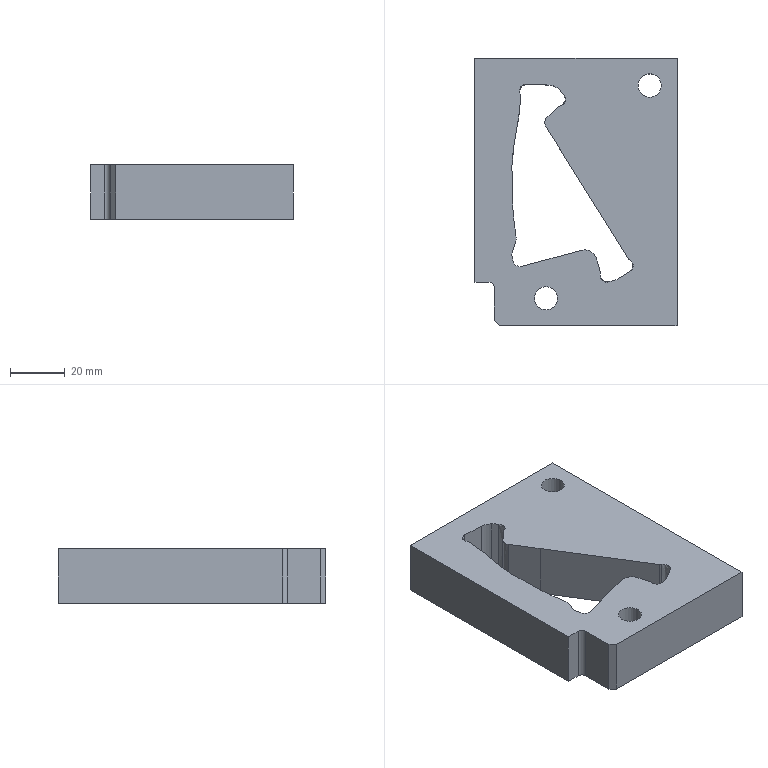Part | NX | features solid 2 | 1 solid | 46 faces | box 74 x 98 x 20 mm | volume 106759 mm3 | spline 18 | plane 16 | cylinder 12 | commonest cylinder face diameters 5 x2 8.5 x2 9 x2 11 x2 14 x2 4 x1